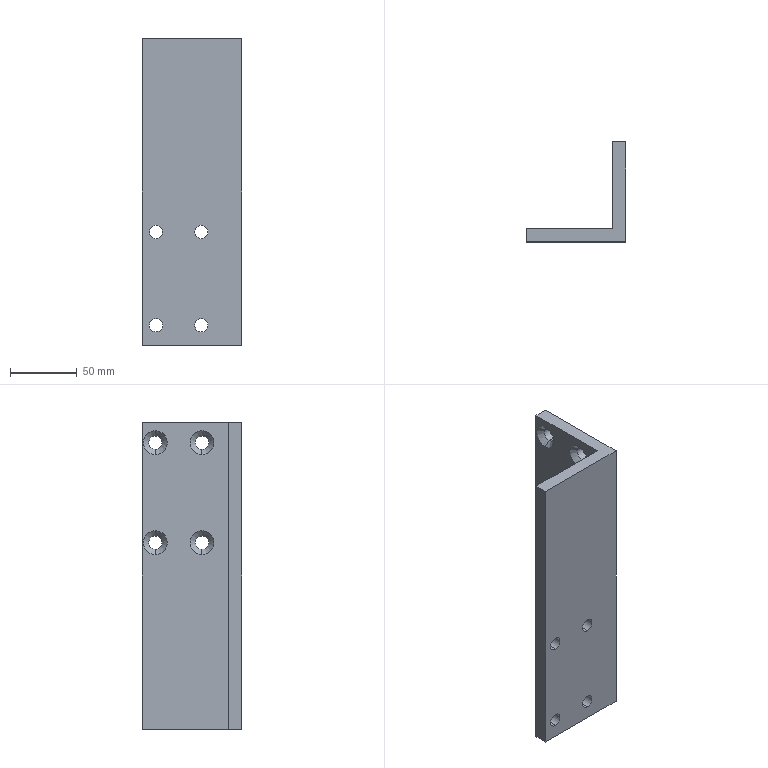Part | SolidWorks | features HoleWzd 2, Extrusion 1, MoveFace 1 | 1 solid | 32 faces | box 75 x 75 x 230 mm | volume 314471 mm3 | cylinder 16 | cone 8 | plane 8 | commonest cylinder face diameters 10 x16
STEP:
#1=CARTESIAN_POINT('',(10.5,0.,-170.));
#2=VERTEX_POINT('',#1);
#3=CARTESIAN_POINT('',(10.5,0.,-160.));
#4=VERTEX_POINT('',#3);
#5=CARTESIAN_POINT('',(10.5,0.,-165.));
#6=DIRECTION('',(0.,1.,0.));
#7=DIRECTION('',(0.,0.,1.));
#8=AXIS2_PLACEMENT_3D('',#5,#6,#7);
#9=CIRCLE('',#8,5.);
#10=EDGE_CURVE('',#2,#4,#9,.T.);
#11=ORIENTED_EDGE('',*,*,#10,.F.);
#12=CARTESIAN_POINT('',(10.5,10.,-170.));
#13=VERTEX_POINT('',#12);
#14=CARTESIAN_POINT('',(10.5,10.,-170.));
#15=DIRECTION('',(0.,1.,0.));
#16=VECTOR('',#15,1000.);
#17=LINE('',#14,#16);
#18=EDGE_CURVE('',#2,#13,#17,.T.);
#19=ORIENTED_EDGE('',*,*,#18,.T.);
#20=CARTESIAN_POINT('',(10.5,10.,-160.));
#21=VERTEX_POINT('',#20);
#22=CARTESIAN_POINT('',(10.5,10.,-165.));
#23=DIRECTION('',(0.,1.,0.));
#24=DIRECTION('',(0.,0.,1.));
#25=AXIS2_PLACEMENT_3D('',#22,#23,#24);
#26=CIRCLE('',#25,5.);
#27=EDGE_CURVE('',#13,#21,#26,.T.);
#28=ORIENTED_EDGE('',*,*,#27,.T.);
#29=CARTESIAN_POINT('',(10.5,10.,-160.));
#30=DIRECTION('',(0.,1.,0.));
#31=VECTOR('',#30,1000.);
#32=LINE('',#29,#31);
#33=EDGE_CURVE('',#4,#21,#32,.T.);
#34=ORIENTED_EDGE('',*,*,#33,.F.);
#35=EDGE_LOOP('',(#11,#19,#28,#34));
#36=FACE_OUTER_BOUND('',#35,.T.);
#37=CARTESIAN_POINT('',(10.5,10.,-165.));
#38=DIRECTION('',(0.,1.,0.));
#39=DIRECTION('',(0.,0.,1.));
#40=AXIS2_PLACEMENT_3D('',#37,#38,#39);
#41=CYLINDRICAL_SURFACE('',#40,5.);
#42=ADVANCED_FACE('',(#36),#41,.F.);
#43=CARTESIAN_POINT('',(10.5,0.,-100.));
#44=VERTEX_POINT('',#43);
#45=CARTESIAN_POINT('',(10.5,0.,-90.));
#46=VERTEX_POINT('',#45);
#47=CARTESIAN_POINT('',(10.5,0.,-95.));
#48=DIRECTION('',(0.,1.,0.));
#49=DIRECTION('',(0.,0.,1.));
#50=AXIS2_PLACEMENT_3D('',#47,#48,#49);
#51=CIRCLE('',#50,5.);
#52=EDGE_CURVE('',#44,#46,#51,.T.);
#53=ORIENTED_EDGE('',*,*,#52,.F.);
#54=CARTESIAN_POINT('',(10.5,10.,-100.));
#55=VERTEX_POINT('',#54);
#56=CARTESIAN_POINT('',(10.5,10.,-100.));
#57=DIRECTION('',(0.,1.,0.));
#58=VECTOR('',#57,1000.);
#59=LINE('',#56,#58);
#60=EDGE_CURVE('',#44,#55,#59,.T.);
#61=ORIENTED_EDGE('',*,*,#60,.T.);
#62=CARTESIAN_POINT('',(10.5,10.,-90.));
#63=VERTEX_POINT('',#62);
#64=CARTESIAN_POINT('',(10.5,10.,-95.));
#65=DIRECTION('',(0.,1.,0.));
#66=DIRECTION('',(0.,0.,1.));
#67=AXIS2_PLACEMENT_3D('',#64,#65,#66);
#68=CIRCLE('',#67,5.);
#69=EDGE_CURVE('',#55,#63,#68,.T.);
#70=ORIENTED_EDGE('',*,*,#69,.T.);
#71=CARTESIAN_POINT('',(10.5,10.,-90.));
#72=DIRECTION('',(0.,1.,0.));
#73=VECTOR('',#72,1000.);
#74=LINE('',#71,#73);
#75=EDGE_CURVE('',#46,#63,#74,.T.);
#76=ORIENTED_EDGE('',*,*,#75,.F.);
#77=EDGE_LOOP('',(#53,#61,#70,#76));
#78=FACE_OUTER_BOUND('',#77,.T.);
#79=CARTESIAN_POINT('',(10.5,10.,-95.));
#80=DIRECTION('',(0.,1.,0.));
#81=DIRECTION('',(0.,0.,1.));
#82=AXIS2_PLACEMENT_3D('',#79,#80,#81);
#83=CYLINDRICAL_SURFACE('',#82,5.);
#84=ADVANCED_FACE('',(#78),#83,.F.);
#85=CARTESIAN_POINT('',(44.5,0.,-170.));
#86=VERTEX_POINT('',#85);
#87=CARTESIAN_POINT('',(44.5,0.,-160.));
#88=VERTEX_POINT('',#87);
#89=CARTESIAN_POINT('',(44.5,0.,-165.));
#90=DIRECTION('',(0.,1.,0.));
#91=DIRECTION('',(0.,0.,1.));
#92=AXIS2_PLACEMENT_3D('',#89,#90,#91);
#93=CIRCLE('',#92,5.);
#94=EDGE_CURVE('',#86,#88,#93,.T.);
#95=ORIENTED_EDGE('',*,*,#94,.F.);
#96=CARTESIAN_POINT('',(44.5,10.,-170.));
#97=VERTEX_POINT('',#96);
#98=CARTESIAN_POINT('',(44.5,10.,-170.));
#99=DIRECTION('',(0.,1.,0.));
#100=VECTOR('',#99,1000.);
#101=LINE('',#98,#100);
#102=EDGE_CURVE('',#86,#97,#101,.T.);
#103=ORIENTED_EDGE('',*,*,#102,.T.);
#104=CARTESIAN_POINT('',(44.5,10.,-160.));
#105=VERTEX_POINT('',#104);
#106=CARTESIAN_POINT('',(44.5,10.,-165.));
#107=DIRECTION('',(0.,1.,0.));
#108=DIRECTION('',(0.,0.,1.));
#109=AXIS2_PLACEMENT_3D('',#106,#107,#108);
#110=CIRCLE('',#109,5.);
#111=EDGE_CURVE('',#97,#105,#110,.T.);
#112=ORIENTED_EDGE('',*,*,#111,.T.);
#113=CARTESIAN_POINT('',(44.5,10.,-160.));
#114=DIRECTION('',(0.,1.,0.));
#115=VECTOR('',#114,1000.);
#116=LINE('',#113,#115);
#117=EDGE_CURVE('',#88,#105,#116,.T.);
#118=ORIENTED_EDGE('',*,*,#117,.F.);
#119=EDGE_LOOP('',(#95,#103,#112,#118));
#120=FACE_OUTER_BOUND('',#119,.T.);
#121=CARTESIAN_POINT('',(44.5,10.,-165.));
#122=DIRECTION('',(0.,1.,0.));
#123=DIRECTION('',(0.,0.,1.));
#124=AXIS2_PLACEMENT_3D('',#121,#122,#123);
#125=CYLINDRICAL_SURFACE('',#124,5.);
#126=ADVANCED_FACE('',(#120),#125,.F.);
#127=CARTESIAN_POINT('',(44.5,0.,-100.));
#128=VERTEX_POINT('',#127);
#129=CARTESIAN_POINT('',(44.5,0.,-90.));
#130=VERTEX_POINT('',#129);
#131=CARTESIAN_POINT('',(44.5,0.,-95.));
#132=DIRECTION('',(0.,1.,0.));
#133=DIRECTION('',(0.,0.,1.));
#134=AXIS2_PLACEMENT_3D('',#131,#132,#133);
#135=CIRCLE('',#134,5.);
#136=EDGE_CURVE('',#128,#130,#135,.T.);
#137=ORIENTED_EDGE('',*,*,#136,.F.);
#138=CARTESIAN_POINT('',(44.5,10.,-100.));
#139=VERTEX_POINT('',#138);
#140=CARTESIAN_POINT('',(44.5,10.,-100.));
#141=DIRECTION('',(0.,1.,0.));
#142=VECTOR('',#141,1000.);
#143=LINE('',#140,#142);
#144=EDGE_CURVE('',#128,#139,#143,.T.);
#145=ORIENTED_EDGE('',*,*,#144,.T.);
#146=CARTESIAN_POINT('',(44.5,10.,-90.));
#147=VERTEX_POINT('',#146);
#148=CARTESIAN_POINT('',(44.5,10.,-95.));
#149=DIRECTION('',(0.,1.,0.));
#150=DIRECTION('',(0.,0.,1.));
#151=AXIS2_PLACEMENT_3D('',#148,#149,#150);
#152=CIRCLE('',#151,5.);
#153=EDGE_CURVE('',#139,#147,#152,.T.);
#154=ORIENTED_EDGE('',*,*,#153,.T.);
#155=CARTESIAN_POINT('',(44.5,10.,-90.));
#156=DIRECTION('',(0.,1.,0.));
#157=VECTOR('',#156,1000.);
#158=LINE('',#155,#157);
#159=EDGE_CURVE('',#130,#147,#158,.T.);
#160=ORIENTED_EDGE('',*,*,#159,.F.);
#161=EDGE_LOOP('',(#137,#145,#154,#160));
#162=FACE_OUTER_BOUND('',#161,.T.);
#163=CARTESIAN_POINT('',(44.5,10.,-95.));
#164=DIRECTION('',(0.,1.,0.));
#165=DIRECTION('',(0.,0.,1.));
#166=AXIS2_PLACEMENT_3D('',#163,#164,#165);
#167=CYLINDRICAL_SURFACE('',#166,5.);
#168=ADVANCED_FACE('',(#162),#167,.F.);
#169=CARTESIAN_POINT('',(68.96,65.,-45.));
#170=VERTEX_POINT('',#169);
#171=CARTESIAN_POINT('',(68.96,65.,-35.));
#172=VERTEX_POINT('',#171);
#173=CARTESIAN_POINT('',(68.96,65.,-40.));
#174=DIRECTION('',(-1.,0.,0.));
#175=DIRECTION('',(0.,0.,1.));
#176=AXIS2_PLACEMENT_3D('',#173,#174,#175);
#177=CIRCLE('',#176,5.);
#178=EDGE_CURVE('',#170,#172,#177,.T.);
#179=ORIENTED_EDGE('',*,*,#178,.F.);
#180=CARTESIAN_POINT('',(65.,65.,-48.96));
#181=VERTEX_POINT('',#180);
#182=CARTESIAN_POINT('',(65.,65.,-48.96));
#183=DIRECTION('',(-0.7071,0.,-0.7071));
#184=VECTOR('',#183,1000.);
#185=LINE('',#182,#184);
#186=EDGE_CURVE('',#170,#181,#185,.T.);
#187=ORIENTED_EDGE('',*,*,#186,.T.);
#188=CARTESIAN_POINT('',(65.,65.,-31.04));
#189=VERTEX_POINT('',#188);
#190=CARTESIAN_POINT('',(65.,65.,-40.));
#191=DIRECTION('',(-1.,0.,0.));
#192=DIRECTION('',(0.,0.,1.));
#193=AXIS2_PLACEMENT_3D('',#190,#191,#192);
#194=CIRCLE('',#193,8.96);
#195=EDGE_CURVE('',#181,#189,#194,.T.);
#196=ORIENTED_EDGE('',*,*,#195,.T.);
#197=CARTESIAN_POINT('',(65.,65.,-31.04));
#198=DIRECTION('',(-0.7071,0.,0.7071));
#199=VECTOR('',#198,1000.);
#200=LINE('',#197,#199);
#201=EDGE_CURVE('',#172,#189,#200,.T.);
#202=ORIENTED_EDGE('',*,*,#201,.F.);
#203=EDGE_LOOP('',(#179,#187,#196,#202));
#204=FACE_OUTER_BOUND('',#203,.T.);
#205=CARTESIAN_POINT('',(65.,65.,-40.));
#206=DIRECTION('',(-1.,0.,0.));
#207=DIRECTION('',(0.,0.,1.));
#208=AXIS2_PLACEMENT_3D('',#205,#206,#207);
#209=CONICAL_SURFACE('',#208,8.96,0.7854);
#210=ADVANCED_FACE('',(#204),#209,.F.);
#211=CARTESIAN_POINT('',(75.,65.,-45.));
#212=VERTEX_POINT('',#211);
#213=CARTESIAN_POINT('',(75.,65.,-35.));
#214=VERTEX_POINT('',#213);
#215=CARTESIAN_POINT('',(75.,65.,-40.));
#216=DIRECTION('',(-1.,0.,0.));
#217=DIRECTION('',(0.,0.,1.));
#218=AXIS2_PLACEMENT_3D('',#215,#216,#217);
#219=CIRCLE('',#218,5.);
#220=EDGE_CURVE('',#212,#214,#219,.T.);
#221=ORIENTED_EDGE('',*,*,#220,.F.);
#222=CARTESIAN_POINT('',(65.,65.,-45.));
#223=DIRECTION('',(-1.,0.,0.));
#224=VECTOR('',#223,1000.);
#225=LINE('',#222,#224);
#226=EDGE_CURVE('',#212,#170,#225,.T.);
#227=ORIENTED_EDGE('',*,*,#226,.T.);
#228=ORIENTED_EDGE('',*,*,#178,.T.);
#229=CARTESIAN_POINT('',(65.,65.,-35.));
#230=DIRECTION('',(-1.,0.,0.));
#231=VECTOR('',#230,1000.);
#232=LINE('',#229,#231);
#233=EDGE_CURVE('',#214,#172,#232,.T.);
#234=ORIENTED_EDGE('',*,*,#233,.F.);
#235=EDGE_LOOP('',(#221,#227,#228,#234));
#236=FACE_OUTER_BOUND('',#235,.T.);
#237=CARTESIAN_POINT('',(65.,65.,-40.));
#238=DIRECTION('',(-1.,0.,0.));
#239=DIRECTION('',(0.,0.,1.));
#240=AXIS2_PLACEMENT_3D('',#237,#238,#239);
#241=CYLINDRICAL_SURFACE('',#240,5.);
#242=ADVANCED_FACE('',(#236),#241,.F.);
#243=CARTESIAN_POINT('',(68.96,65.,30.));
#244=VERTEX_POINT('',#243);
#245=CARTESIAN_POINT('',(68.96,65.,40.));
#246=VERTEX_POINT('',#245);
#247=CARTESIAN_POINT('',(68.96,65.,35.));
#248=DIRECTION('',(-1.,0.,0.));
#249=DIRECTION('',(0.,0.,1.));
#250=AXIS2_PLACEMENT_3D('',#247,#248,#249);
#251=CIRCLE('',#250,5.);
#252=EDGE_CURVE('',#244,#246,#251,.T.);
#253=ORIENTED_EDGE('',*,*,#252,.F.);
#254=CARTESIAN_POINT('',(65.,65.,26.04));
#255=VERTEX_POINT('',#254);
#256=CARTESIAN_POINT('',(65.,65.,26.04));
#257=DIRECTION('',(-0.7071,0.,-0.7071));
#258=VECTOR('',#257,1000.);
#259=LINE('',#256,#258);
#260=EDGE_CURVE('',#244,#255,#259,.T.);
#261=ORIENTED_EDGE('',*,*,#260,.T.);
#262=CARTESIAN_POINT('',(65.,65.,43.96));
#263=VERTEX_POINT('',#262);
#264=CARTESIAN_POINT('',(65.,65.,35.));
#265=DIRECTION('',(-1.,0.,0.));
#266=DIRECTION('',(0.,0.,1.));
#267=AXIS2_PLACEMENT_3D('',#264,#265,#266);
#268=CIRCLE('',#267,8.96);
#269=EDGE_CURVE('',#255,#263,#268,.T.);
#270=ORIENTED_EDGE('',*,*,#269,.T.);
#271=CARTESIAN_POINT('',(65.,65.,43.96));
#272=DIRECTION('',(-0.7071,0.,0.7071));
#273=VECTOR('',#272,1000.);
#274=LINE('',#271,#273);
#275=EDGE_CURVE('',#246,#263,#274,.T.);
#276=ORIENTED_EDGE('',*,*,#275,.F.);
#277=EDGE_LOOP('',(#253,#261,#270,#276));
#278=FACE_OUTER_BOUND('',#277,.T.);
#279=CARTESIAN_POINT('',(65.,65.,35.));
#280=DIRECTION('',(-1.,0.,0.));
#281=DIRECTION('',(0.,0.,1.));
#282=AXIS2_PLACEMENT_3D('',#279,#280,#281);
#283=CONICAL_SURFACE('',#282,8.96,0.7854);
#284=ADVANCED_FACE('',(#278),#283,.F.);
#285=CARTESIAN_POINT('',(75.,65.,30.));
#286=VERTEX_POINT('',#285);
#287=CARTESIAN_POINT('',(75.,65.,40.));
#288=VERTEX_POINT('',#287);
#289=CARTESIAN_POINT('',(75.,65.,35.));
#290=DIRECTION('',(-1.,0.,0.));
#291=DIRECTION('',(0.,0.,1.));
#292=AXIS2_PLACEMENT_3D('',#289,#290,#291);
#293=CIRCLE('',#292,5.);
#294=EDGE_CURVE('',#286,#288,#293,.T.);
#295=ORIENTED_EDGE('',*,*,#294,.F.);
#296=CARTESIAN_POINT('',(65.,65.,30.));
#297=DIRECTION('',(-1.,0.,0.));
#298=VECTOR('',#297,1000.);
#299=LINE('',#296,#298);
#300=EDGE_CURVE('',#286,#244,#299,.T.);
#301=ORIENTED_EDGE('',*,*,#300,.T.);
#302=ORIENTED_EDGE('',*,*,#252,.T.);
#303=CARTESIAN_POINT('',(65.,65.,40.));
#304=DIRECTION('',(-1.,0.,0.));
#305=VECTOR('',#304,1000.);
#306=LINE('',#303,#305);
#307=EDGE_CURVE('',#288,#246,#306,.T.);
#308=ORIENTED_EDGE('',*,*,#307,.F.);
#309=EDGE_LOOP('',(#295,#301,#302,#308));
#310=FACE_OUTER_BOUND('',#309,.T.);
#311=CARTESIAN_POINT('',(65.,65.,35.));
#312=DIRECTION('',(-1.,0.,0.));
#313=DIRECTION('',(0.,0.,1.));
#314=AXIS2_PLACEMENT_3D('',#311,#312,#313);
#315=CYLINDRICAL_SURFACE('',#314,5.);
#316=ADVANCED_FACE('',(#310),#315,.F.);
#317=CARTESIAN_POINT('',(68.96,30.,-45.));
#318=VERTEX_POINT('',#317);
#319=CARTESIAN_POINT('',(68.96,30.,-35.));
#320=VERTEX_POINT('',#319);
#321=CARTESIAN_POINT('',(68.96,30.,-40.));
#322=DIRECTION('',(-1.,0.,0.));
#323=DIRECTION('',(0.,0.,1.));
#324=AXIS2_PLACEMENT_3D('',#321,#322,#323);
#325=CIRCLE('',#324,5.);
#326=EDGE_CURVE('',#318,#320,#325,.T.);
#327=ORIENTED_EDGE('',*,*,#326,.F.);
#328=CARTESIAN_POINT('',(65.,30.,-48.96));
#329=VERTEX_POINT('',#328);
#330=CARTESIAN_POINT('',(65.,30.,-48.96));
#331=DIRECTION('',(-0.7071,0.,-0.7071));
#332=VECTOR('',#331,1000.);
#333=LINE('',#330,#332);
#334=EDGE_CURVE('',#318,#329,#333,.T.);
#335=ORIENTED_EDGE('',*,*,#334,.T.);
#336=CARTESIAN_POINT('',(65.,30.,-31.04));
#337=VERTEX_POINT('',#336);
#338=CARTESIAN_POINT('',(65.,30.,-40.));
#339=DIRECTION('',(-1.,0.,0.));
#340=DIRECTION('',(0.,0.,1.));
#341=AXIS2_PLACEMENT_3D('',#338,#339,#340);
#342=CIRCLE('',#341,8.96);
#343=EDGE_CURVE('',#329,#337,#342,.T.);
#344=ORIENTED_EDGE('',*,*,#343,.T.);
#345=CARTESIAN_POINT('',(65.,30.,-31.04));
#346=DIRECTION('',(-0.7071,0.,0.7071));
#347=VECTOR('',#346,1000.);
#348=LINE('',#345,#347);
#349=EDGE_CURVE('',#320,#337,#348,.T.);
#350=ORIENTED_EDGE('',*,*,#349,.F.);
#351=EDGE_LOOP('',(#327,#335,#344,#350));
#352=FACE_OUTER_BOUND('',#351,.T.);
#353=CARTESIAN_POINT('',(65.,30.,-40.));
#354=DIRECTION('',(-1.,0.,0.));
#355=DIRECTION('',(0.,0.,1.));
#356=AXIS2_PLACEMENT_3D('',#353,#354,#355);
#357=CONICAL_SURFACE('',#356,8.96,0.7854);
#358=ADVANCED_FACE('',(#352),#357,.F.);
#359=CARTESIAN_POINT('',(75.,30.,-45.));
#360=VERTEX_POINT('',#359);
#361=CARTESIAN_POINT('',(75.,30.,-35.));
#362=VERTEX_POINT('',#361);
#363=CARTESIAN_POINT('',(75.,30.,-40.));
#364=DIRECTION('',(-1.,0.,0.));
#365=DIRECTION('',(0.,0.,1.));
#366=AXIS2_PLACEMENT_3D('',#363,#364,#365);
#367=CIRCLE('',#366,5.);
#368=EDGE_CURVE('',#360,#362,#367,.T.);
#369=ORIENTED_EDGE('',*,*,#368,.F.);
#370=CARTESIAN_POINT('',(65.,30.,-45.));
#371=DIRECTION('',(-1.,0.,0.));
#372=VECTOR('',#371,1000.);
#373=LINE('',#370,#372);
#374=EDGE_CURVE('',#360,#318,#373,.T.);
#375=ORIENTED_EDGE('',*,*,#374,.T.);
#376=ORIENTED_EDGE('',*,*,#326,.T.);
#377=CARTESIAN_POINT('',(65.,30.,-35.));
#378=DIRECTION('',(-1.,0.,0.));
#379=VECTOR('',#378,1000.);
#380=LINE('',#377,#379);
#381=EDGE_CURVE('',#362,#320,#380,.T.);
#382=ORIENTED_EDGE('',*,*,#381,.F.);
#383=EDGE_LOOP('',(#369,#375,#376,#382));
#384=FACE_OUTER_BOUND('',#383,.T.);
#385=CARTESIAN_POINT('',(65.,30.,-40.));
#386=DIRECTION('',(-1.,0.,0.));
#387=DIRECTION('',(0.,0.,1.));
#388=AXIS2_PLACEMENT_3D('',#385,#386,#387);
#389=CYLINDRICAL_SURFACE('',#388,5.);
#390=ADVANCED_FACE('',(#384),#389,.F.);
#391=CARTESIAN_POINT('',(68.96,30.,30.));
#392=VERTEX_POINT('',#391);
#393=CARTESIAN_POINT('',(68.96,30.,40.));
#394=VERTEX_POINT('',#393);
#395=CARTESIAN_POINT('',(68.96,30.,35.));
#396=DIRECTION('',(-1.,0.,0.));
#397=DIRECTION('',(0.,0.,1.));
#398=AXIS2_PLACEMENT_3D('',#395,#396,#397);
#399=CIRCLE('',#398,5.);
#400=EDGE_CURVE('',#392,#394,#399,.T.);
#401=ORIENTED_EDGE('',*,*,#400,.F.);
#402=CARTESIAN_POINT('',(65.,30.,26.04));
#403=VERTEX_POINT('',#402);
#404=CARTESIAN_POINT('',(65.,30.,26.04));
#405=DIRECTION('',(-0.7071,0.,-0.7071));
#406=VECTOR('',#405,1000.);
#407=LINE('',#404,#406);
#408=EDGE_CURVE('',#392,#403,#407,.T.);
#409=ORIENTED_EDGE('',*,*,#408,.T.);
#410=CARTESIAN_POINT('',(65.,30.,43.96));
#411=VERTEX_POINT('',#410);
#412=CARTESIAN_POINT('',(65.,30.,35.));
#413=DIRECTION('',(-1.,0.,0.));
#414=DIRECTION('',(0.,0.,1.));
#415=AXIS2_PLACEMENT_3D('',#412,#413,#414);
#416=CIRCLE('',#415,8.96);
#417=EDGE_CURVE('',#403,#411,#416,.T.);
#418=ORIENTED_EDGE('',*,*,#417,.T.);
#419=CARTESIAN_POINT('',(65.,30.,43.96));
#420=DIRECTION('',(-0.7071,0.,0.7071));
#421=VECTOR('',#420,1000.);
#422=LINE('',#419,#421);
#423=EDGE_CURVE('',#394,#411,#422,.T.);
#424=ORIENTED_EDGE('',*,*,#423,.F.);
#425=EDGE_LOOP('',(#401,#409,#418,#424));
#426=FACE_OUTER_BOUND('',#425,.T.);
#427=CARTESIAN_POINT('',(65.,30.,35.));
#428=DIRECTION('',(-1.,0.,0.));
#429=DIRECTION('',(0.,0.,1.));
#430=AXIS2_PLACEMENT_3D('',#427,#428,#429);
#431=CONICAL_SURFACE('',#430,8.96,0.7854);
#432=ADVANCED_FACE('',(#426),#431,.F.);
#433=CARTESIAN_POINT('',(75.,30.,30.));
#434=VERTEX_POINT('',#433);
#435=CARTESIAN_POINT('',(75.,30.,40.));
#436=VERTEX_POINT('',#435);
#437=CARTESIAN_POINT('',(75.,30.,35.));
#438=DIRECTION('',(-1.,0.,0.));
#439=DIRECTION('',(0.,0.,1.));
#440=AXIS2_PLACEMENT_3D('',#437,#438,#439);
#441=CIRCLE('',#440,5.);
#442=EDGE_CURVE('',#434,#436,#441,.T.);
#443=ORIENTED_EDGE('',*,*,#442,.F.);
#444=CARTESIAN_POINT('',(65.,30.,30.));
#445=DIRECTION('',(-1.,0.,0.));
#446=VECTOR('',#445,1000.);
#447=LINE('',#444,#446);
#448=EDGE_CURVE('',#434,#392,#447,.T.);
#449=ORIENTED_EDGE('',*,*,#448,.T.);
#450=ORIENTED_EDGE('',*,*,#400,.T.);
#451=CARTESIAN_POINT('',(65.,30.,40.));
#452=DIRECTION('',(-1.,0.,0.));
#453=VECTOR('',#452,1000.);
#454=LINE('',#451,#453);
#455=EDGE_CURVE('',#436,#394,#454,.T.);
#456=ORIENTED_EDGE('',*,*,#455,.F.);
#457=EDGE_LOOP('',(#443,#449,#450,#456));
#458=FACE_OUTER_BOUND('',#457,.T.);
#459=CARTESIAN_POINT('',(65.,30.,35.));
#460=DIRECTION('',(-1.,0.,0.));
#461=DIRECTION('',(0.,0.,1.));
#462=AXIS2_PLACEMENT_3D('',#459,#460,#461);
#463=CYLINDRICAL_SURFACE('',#462,5.);
#464=ADVANCED_FACE('',(#458),#463,.F.);
#465=CARTESIAN_POINT('',(10.5,10.,-165.));
#466=DIRECTION('',(0.,1.,0.));
#467=DIRECTION('',(0.,0.,1.));
#468=AXIS2_PLACEMENT_3D('',#465,#466,#467);
#469=CIRCLE('',#468,5.);
#470=EDGE_CURVE('',#21,#13,#469,.T.);
#471=ORIENTED_EDGE('',*,*,#470,.F.);
#472=ORIENTED_EDGE('',*,*,#27,.F.);
#473=EDGE_LOOP('',(#471,#472));
#474=FACE_BOUND('',#473,.T.);
#475=CARTESIAN_POINT('',(10.5,10.,-95.));
#476=DIRECTION('',(0.,1.,0.));
#477=DIRECTION('',(0.,0.,1.));
#478=AXIS2_PLACEMENT_3D('',#475,#476,#477);
#479=CIRCLE('',#478,5.);
#480=EDGE_CURVE('',#63,#55,#479,.T.);
#481=ORIENTED_EDGE('',*,*,#480,.F.);
#482=ORIENTED_EDGE('',*,*,#69,.F.);
#483=EDGE_LOOP('',(#481,#482));
#484=FACE_BOUND('',#483,.T.);
#485=CARTESIAN_POINT('',(44.5,10.,-165.));
#486=DIRECTION('',(0.,1.,0.));
#487=DIRECTION('',(0.,0.,1.));
#488=AXIS2_PLACEMENT_3D('',#485,#486,#487);
#489=CIRCLE('',#488,5.);
#490=EDGE_CURVE('',#105,#97,#489,.T.);
#491=ORIENTED_EDGE('',*,*,#490,.F.);
#492=ORIENTED_EDGE('',*,*,#111,.F.);
#493=EDGE_LOOP('',(#491,#492));
#494=FACE_BOUND('',#493,.T.);
#495=CARTESIAN_POINT('',(65.,10.,-180.));
#496=VERTEX_POINT('',#495);
#497=CARTESIAN_POINT('',(0.,10.,-180.));
#498=VERTEX_POINT('',#497);
#499=CARTESIAN_POINT('',(65.,10.,-180.));
#500=DIRECTION('',(-1.,0.,0.));
#501=VECTOR('',#500,1000.);
#502=LINE('',#499,#501);
#503=EDGE_CURVE('',#496,#498,#502,.T.);
#504=ORIENTED_EDGE('',*,*,#503,.T.);
#505=CARTESIAN_POINT('',(0.,10.,50.));
#506=VERTEX_POINT('',#505);
#507=CARTESIAN_POINT('',(0.,10.,50.));
#508=DIRECTION('',(0.,0.,-1.));
#509=VECTOR('',#508,1000.);
#510=LINE('',#507,#509);
#511=EDGE_CURVE('',#506,#498,#510,.T.);
#512=ORIENTED_EDGE('',*,*,#511,.F.);
#513=CARTESIAN_POINT('',(65.,10.,50.));
#514=VERTEX_POINT('',#513);
#515=CARTESIAN_POINT('',(65.,10.,50.));
#516=DIRECTION('',(-1.,0.,0.));
#517=VECTOR('',#516,1000.);
#518=LINE('',#515,#517);
#519=EDGE_CURVE('',#514,#506,#518,.T.);
#520=ORIENTED_EDGE('',*,*,#519,.F.);
#521=CARTESIAN_POINT('',(65.,10.,50.));
#522=DIRECTION('',(0.,0.,-1.));
#523=VECTOR('',#522,1000.);
#524=LINE('',#521,#523);
#525=EDGE_CURVE('',#514,#496,#524,.T.);
#526=ORIENTED_EDGE('',*,*,#525,.T.);
#527=EDGE_LOOP('',(#504,#512,#520,#526));
#528=FACE_OUTER_BOUND('',#527,.T.);
#529=CARTESIAN_POINT('',(44.5,10.,-95.));
#530=DIRECTION('',(0.,1.,0.));
#531=DIRECTION('',(0.,0.,1.));
#532=AXIS2_PLACEMENT_3D('',#529,#530,#531);
#533=CIRCLE('',#532,5.);
#534=EDGE_CURVE('',#147,#139,#533,.T.);
#535=ORIENTED_EDGE('',*,*,#534,.F.);
#536=ORIENTED_EDGE('',*,*,#153,.F.);
#537=EDGE_LOOP('',(#535,#536));
#538=FACE_BOUND('',#537,.T.);
#539=CARTESIAN_POINT('',(65.,10.,50.));
#540=DIRECTION('',(0.,-1.,0.));
#541=DIRECTION('',(1.,0.,0.));
#542=AXIS2_PLACEMENT_3D('',#539,#540,#541);
#543=PLANE('',#542);
#544=ADVANCED_FACE('',(#474,#484,#494,#528,#538),#543,.F.);
#545=CARTESIAN_POINT('',(0.,0.,-180.));
#546=VERTEX_POINT('',#545);
#547=CARTESIAN_POINT('',(0.,10.,-180.));
#548=DIRECTION('',(0.,-1.,0.));
#549=VECTOR('',#548,1000.);
#550=LINE('',#547,#549);
#551=EDGE_CURVE('',#498,#546,#550,.T.);
#552=ORIENTED_EDGE('',*,*,#551,.T.);
#553=CARTESIAN_POINT('',(0.,0.,50.));
#554=VERTEX_POINT('',#553);
#555=CARTESIAN_POINT('',(0.,0.,50.));
#556=DIRECTION('',(0.,0.,-1.));
#557=VECTOR('',#556,1000.);
#558=LINE('',#555,#557);
#559=EDGE_CURVE('',#554,#546,#558,.T.);
#560=ORIENTED_EDGE('',*,*,#559,.F.);
#561=CARTESIAN_POINT('',(0.,10.,50.));
#562=DIRECTION('',(0.,-1.,0.));
#563=VECTOR('',#562,1000.);
#564=LINE('',#561,#563);
#565=EDGE_CURVE('',#506,#554,#564,.T.);
#566=ORIENTED_EDGE('',*,*,#565,.F.);
#567=ORIENTED_EDGE('',*,*,#511,.T.);
#568=EDGE_LOOP('',(#552,#560,#566,#567));
#569=FACE_OUTER_BOUND('',#568,.T.);
#570=CARTESIAN_POINT('',(0.,10.,50.));
#571=DIRECTION('',(1.,0.,0.));
#572=DIRECTION('',(0.,1.,0.));
#573=AXIS2_PLACEMENT_3D('',#570,#571,#572);
#574=PLANE('',#573);
#575=ADVANCED_FACE('',(#569),#574,.F.);
#576=CARTESIAN_POINT('',(10.5,0.,-165.));
#577=DIRECTION('',(0.,1.,0.));
#578=DIRECTION('',(0.,0.,1.));
#579=AXIS2_PLACEMENT_3D('',#576,#577,#578);
#580=CIRCLE('',#579,5.);
#581=EDGE_CURVE('',#4,#2,#580,.T.);
#582=ORIENTED_EDGE('',*,*,#581,.T.);
#583=ORIENTED_EDGE('',*,*,#10,.T.);
#584=EDGE_LOOP('',(#582,#583));
#585=FACE_BOUND('',#584,.T.);
#586=CARTESIAN_POINT('',(10.5,0.,-95.));
#587=DIRECTION('',(0.,1.,0.));
#588=DIRECTION('',(0.,0.,1.));
#589=AXIS2_PLACEMENT_3D('',#586,#587,#588);
#590=CIRCLE('',#589,5.);
#591=EDGE_CURVE('',#46,#44,#590,.T.);
#592=ORIENTED_EDGE('',*,*,#591,.T.);
#593=ORIENTED_EDGE('',*,*,#52,.T.);
#594=EDGE_LOOP('',(#592,#593));
#595=FACE_BOUND('',#594,.T.);
#596=CARTESIAN_POINT('',(44.5,0.,-165.));
#597=DIRECTION('',(0.,1.,0.));
#598=DIRECTION('',(0.,0.,1.));
#599=AXIS2_PLACEMENT_3D('',#596,#597,#598);
#600=CIRCLE('',#599,5.);
#601=EDGE_CURVE('',#88,#86,#600,.T.);
#602=ORIENTED_EDGE('',*,*,#601,.T.);
#603=ORIENTED_EDGE('',*,*,#94,.T.);
#604=EDGE_LOOP('',(#602,#603));
#605=FACE_BOUND('',#604,.T.);
#606=CARTESIAN_POINT('',(44.5,0.,-95.));
#607=DIRECTION('',(0.,1.,0.));
#608=DIRECTION('',(0.,0.,1.));
#609=AXIS2_PLACEMENT_3D('',#606,#607,#608);
#610=CIRCLE('',#609,5.);
#611=EDGE_CURVE('',#130,#128,#610,.T.);
#612=ORIENTED_EDGE('',*,*,#611,.T.);
#613=ORIENTED_EDGE('',*,*,#136,.T.);
#614=EDGE_LOOP('',(#612,#613));
#615=FACE_BOUND('',#614,.T.);
#616=CARTESIAN_POINT('',(75.,0.,-180.));
#617=VERTEX_POINT('',#616);
#618=CARTESIAN_POINT('',(0.,0.,-180.));
#619=DIRECTION('',(1.,0.,0.));
#620=VECTOR('',#619,1000.);
#621=LINE('',#618,#620);
#622=EDGE_CURVE('',#546,#617,#621,.T.);
#623=ORIENTED_EDGE('',*,*,#622,.T.);
#624=CARTESIAN_POINT('',(75.,0.,50.));
#625=VERTEX_POINT('',#624);
#626=CARTESIAN_POINT('',(75.,0.,50.));
#627=DIRECTION('',(0.,0.,-1.));
#628=VECTOR('',#627,1000.);
#629=LINE('',#626,#628);
#630=EDGE_CURVE('',#625,#617,#629,.T.);
#631=ORIENTED_EDGE('',*,*,#630,.F.);
#632=CARTESIAN_POINT('',(0.,0.,50.));
#633=DIRECTION('',(1.,0.,0.));
#634=VECTOR('',#633,1000.);
#635=LINE('',#632,#634);
#636=EDGE_CURVE('',#554,#625,#635,.T.);
#637=ORIENTED_EDGE('',*,*,#636,.F.);
#638=ORIENTED_EDGE('',*,*,#559,.T.);
#639=EDGE_LOOP('',(#623,#631,#637,#638));
#640=FACE_OUTER_BOUND('',#639,.T.);
#641=CARTESIAN_POINT('',(0.,0.,50.));
#642=DIRECTION('',(0.,1.,0.));
#643=DIRECTION('',(0.,0.,1.));
#644=AXIS2_PLACEMENT_3D('',#641,#642,#643);
#645=PLANE('',#644);
#646=ADVANCED_FACE('',(#585,#595,#605,#615,#640),#645,.F.);
#647=CARTESIAN_POINT('',(75.,65.,-40.));
#648=DIRECTION('',(-1.,0.,0.));
#649=DIRECTION('',(0.,0.,1.));
#650=AXIS2_PLACEMENT_3D('',#647,#648,#649);
#651=CIRCLE('',#650,5.);
#652=EDGE_CURVE('',#214,#212,#651,.T.);
#653=ORIENTED_EDGE('',*,*,#652,.T.);
#654=ORIENTED_EDGE('',*,*,#220,.T.);
#655=EDGE_LOOP('',(#653,#654));
#656=FACE_BOUND('',#655,.T.);
#657=CARTESIAN_POINT('',(75.,65.,35.));
#658=DIRECTION('',(-1.,0.,0.));
#659=DIRECTION('',(0.,0.,1.));
#660=AXIS2_PLACEMENT_3D('',#657,#658,#659);
#661=CIRCLE('',#660,5.);
#662=EDGE_CURVE('',#288,#286,#661,.T.);
#663=ORIENTED_EDGE('',*,*,#662,.T.);
#664=ORIENTED_EDGE('',*,*,#294,.T.);
#665=EDGE_LOOP('',(#663,#664));
#666=FACE_BOUND('',#665,.T.);
#667=CARTESIAN_POINT('',(75.,30.,-40.));
#668=DIRECTION('',(-1.,0.,0.));
#669=DIRECTION('',(0.,0.,1.));
#670=AXIS2_PLACEMENT_3D('',#667,#668,#669);
#671=CIRCLE('',#670,5.);
#672=EDGE_CURVE('',#362,#360,#671,.T.);
#673=ORIENTED_EDGE('',*,*,#672,.T.);
#674=ORIENTED_EDGE('',*,*,#368,.T.);
#675=EDGE_LOOP('',(#673,#674));
#676=FACE_BOUND('',#675,.T.);
#677=CARTESIAN_POINT('',(75.,30.,35.));
#678=DIRECTION('',(-1.,0.,0.));
#679=DIRECTION('',(0.,0.,1.));
#680=AXIS2_PLACEMENT_3D('',#677,#678,#679);
#681=CIRCLE('',#680,5.);
#682=EDGE_CURVE('',#436,#434,#681,.T.);
#683=ORIENTED_EDGE('',*,*,#682,.T.);
#684=ORIENTED_EDGE('',*,*,#442,.T.);
#685=EDGE_LOOP('',(#683,#684));
#686=FACE_BOUND('',#685,.T.);
#687=CARTESIAN_POINT('',(75.,75.,-180.));
#688=VERTEX_POINT('',#687);
#689=CARTESIAN_POINT('',(75.,0.,-180.));
#690=DIRECTION('',(0.,1.,0.));
#691=VECTOR('',#690,1000.);
#692=LINE('',#689,#691);
#693=EDGE_CURVE('',#617,#688,#692,.T.);
#694=ORIENTED_EDGE('',*,*,#693,.T.);
#695=CARTESIAN_POINT('',(75.,75.,50.));
#696=VERTEX_POINT('',#695);
#697=CARTESIAN_POINT('',(75.,75.,50.));
#698=DIRECTION('',(0.,0.,-1.));
#699=VECTOR('',#698,1000.);
#700=LINE('',#697,#699);
#701=EDGE_CURVE('',#696,#688,#700,.T.);
#702=ORIENTED_EDGE('',*,*,#701,.F.);
#703=CARTESIAN_POINT('',(75.,0.,50.));
#704=DIRECTION('',(0.,1.,0.));
#705=VECTOR('',#704,1000.);
#706=LINE('',#703,#705);
#707=EDGE_CURVE('',#625,#696,#706,.T.);
#708=ORIENTED_EDGE('',*,*,#707,.F.);
#709=ORIENTED_EDGE('',*,*,#630,.T.);
#710=EDGE_LOOP('',(#694,#702,#708,#709));
#711=FACE_OUTER_BOUND('',#710,.T.);
#712=CARTESIAN_POINT('',(75.,0.,50.));
#713=DIRECTION('',(-1.,0.,0.));
#714=DIRECTION('',(0.,0.,1.));
#715=AXIS2_PLACEMENT_3D('',#712,#713,#714);
#716=PLANE('',#715);
#717=ADVANCED_FACE('',(#656,#666,#676,#686,#711),#716,.F.);
#718=CARTESIAN_POINT('',(65.,75.,-180.));
#719=VERTEX_POINT('',#718);
#720=CARTESIAN_POINT('',(75.,75.,-180.));
#721=DIRECTION('',(-1.,0.,0.));
#722=VECTOR('',#721,1000.);
#723=LINE('',#720,#722);
#724=EDGE_CURVE('',#688,#719,#723,.T.);
#725=ORIENTED_EDGE('',*,*,#724,.T.);
#726=CARTESIAN_POINT('',(65.,75.,50.));
#727=VERTEX_POINT('',#726);
#728=CARTESIAN_POINT('',(65.,75.,50.));
#729=DIRECTION('',(0.,0.,-1.));
#730=VECTOR('',#729,1000.);
#731=LINE('',#728,#730);
#732=EDGE_CURVE('',#727,#719,#731,.T.);
#733=ORIENTED_EDGE('',*,*,#732,.F.);
#734=CARTESIAN_POINT('',(75.,75.,50.));
#735=DIRECTION('',(-1.,0.,0.));
#736=VECTOR('',#735,1000.);
#737=LINE('',#734,#736);
#738=EDGE_CURVE('',#696,#727,#737,.T.);
#739=ORIENTED_EDGE('',*,*,#738,.F.);
#740=ORIENTED_EDGE('',*,*,#701,.T.);
#741=EDGE_LOOP('',(#725,#733,#739,#740));
#742=FACE_OUTER_BOUND('',#741,.T.);
#743=CARTESIAN_POINT('',(75.,75.,50.));
#744=DIRECTION('',(0.,-1.,0.));
#745=DIRECTION('',(0.,0.,-1.));
#746=AXIS2_PLACEMENT_3D('',#743,#744,#745);
#747=PLANE('',#746);
#748=ADVANCED_FACE('',(#742),#747,.F.);
#749=CARTESIAN_POINT('',(65.,65.,-40.));
#750=DIRECTION('',(-1.,0.,0.));
#751=DIRECTION('',(0.,0.,1.));
#752=AXIS2_PLACEMENT_3D('',#749,#750,#751);
#753=CIRCLE('',#752,8.96);
#754=EDGE_CURVE('',#189,#181,#753,.T.);
#755=ORIENTED_EDGE('',*,*,#754,.F.);
#756=ORIENTED_EDGE('',*,*,#195,.F.);
#757=EDGE_LOOP('',(#755,#756));
#758=FACE_BOUND('',#757,.T.);
#759=CARTESIAN_POINT('',(65.,65.,35.));
#760=DIRECTION('',(-1.,0.,0.));
#761=DIRECTION('',(0.,0.,1.));
#762=AXIS2_PLACEMENT_3D('',#759,#760,#761);
#763=CIRCLE('',#762,8.96);
#764=EDGE_CURVE('',#263,#255,#763,.T.);
#765=ORIENTED_EDGE('',*,*,#764,.F.);
#766=ORIENTED_EDGE('',*,*,#269,.F.);
#767=EDGE_LOOP('',(#765,#766));
#768=FACE_BOUND('',#767,.T.);
#769=CARTESIAN_POINT('',(65.,30.,-40.));
#770=DIRECTION('',(-1.,0.,0.));
#771=DIRECTION('',(0.,0.,1.));
#772=AXIS2_PLACEMENT_3D('',#769,#770,#771);
#773=CIRCLE('',#772,8.96);
#774=EDGE_CURVE('',#337,#329,#773,.T.);
#775=ORIENTED_EDGE('',*,*,#774,.F.);
#776=ORIENTED_EDGE('',*,*,#343,.F.);
#777=EDGE_LOOP('',(#775,#776));
#778=FACE_BOUND('',#777,.T.);
#779=CARTESIAN_POINT('',(65.,30.,35.));
#780=DIRECTION('',(-1.,0.,0.));
#781=DIRECTION('',(0.,0.,1.));
#782=AXIS2_PLACEMENT_3D('',#779,#780,#781);
#783=CIRCLE('',#782,8.96);
#784=EDGE_CURVE('',#411,#403,#783,.T.);
#785=ORIENTED_EDGE('',*,*,#784,.F.);
#786=ORIENTED_EDGE('',*,*,#417,.F.);
#787=EDGE_LOOP('',(#785,#786));
#788=FACE_BOUND('',#787,.T.);
#789=CARTESIAN_POINT('',(65.,75.,-180.));
#790=DIRECTION('',(0.,-1.,0.));
#791=VECTOR('',#790,1000.);
#792=LINE('',#789,#791);
#793=EDGE_CURVE('',#719,#496,#792,.T.);
#794=ORIENTED_EDGE('',*,*,#793,.T.);
#795=ORIENTED_EDGE('',*,*,#525,.F.);
#796=CARTESIAN_POINT('',(65.,75.,50.));
#797=DIRECTION('',(0.,-1.,0.));
#798=VECTOR('',#797,1000.);
#799=LINE('',#796,#798);
#800=EDGE_CURVE('',#727,#514,#799,.T.);
#801=ORIENTED_EDGE('',*,*,#800,.F.);
#802=ORIENTED_EDGE('',*,*,#732,.T.);
#803=EDGE_LOOP('',(#794,#795,#801,#802));
#804=FACE_OUTER_BOUND('',#803,.T.);
#805=CARTESIAN_POINT('',(65.,75.,50.));
#806=DIRECTION('',(1.,0.,0.));
#807=DIRECTION('',(0.,0.,-1.));
#808=AXIS2_PLACEMENT_3D('',#805,#806,#807);
#809=PLANE('',#808);
#810=ADVANCED_FACE('',(#758,#768,#778,#788,#804),#809,.F.);
#811=ORIENTED_EDGE('',*,*,#565,.T.);
#812=ORIENTED_EDGE('',*,*,#636,.T.);
#813=ORIENTED_EDGE('',*,*,#707,.T.);
#814=ORIENTED_EDGE('',*,*,#738,.T.);
#815=ORIENTED_EDGE('',*,*,#800,.T.);
#816=ORIENTED_EDGE('',*,*,#519,.T.);
#817=EDGE_LOOP('',(#811,#812,#813,#814,#815,#816));
#818=FACE_OUTER_BOUND('',#817,.T.);
#819=CARTESIAN_POINT('',(0.,0.,50.));
#820=DIRECTION('',(0.,0.,1.));
#821=DIRECTION('',(1.,0.,0.));
#822=AXIS2_PLACEMENT_3D('',#819,#820,#821);
#823=PLANE('',#822);
#824=ADVANCED_FACE('',(#818),#823,.T.);
#825=ORIENTED_EDGE('',*,*,#551,.F.);
#826=ORIENTED_EDGE('',*,*,#503,.F.);
#827=ORIENTED_EDGE('',*,*,#793,.F.);
#828=ORIENTED_EDGE('',*,*,#724,.F.);
#829=ORIENTED_EDGE('',*,*,#693,.F.);
#830=ORIENTED_EDGE('',*,*,#622,.F.);
#831=EDGE_LOOP('',(#825,#826,#827,#828,#829,#830));
#832=FACE_OUTER_BOUND('',#831,.T.);
#833=CARTESIAN_POINT('',(0.,0.,-180.));
#834=DIRECTION('',(0.,0.,1.));
#835=DIRECTION('',(1.,0.,0.));
#836=AXIS2_PLACEMENT_3D('',#833,#834,#835);
#837=PLANE('',#836);
#838=ADVANCED_FACE('',(#832),#837,.F.);
#839=ORIENTED_EDGE('',*,*,#448,.F.);
#840=ORIENTED_EDGE('',*,*,#682,.F.);
#841=ORIENTED_EDGE('',*,*,#455,.T.);
#842=CARTESIAN_POINT('',(68.96,30.,35.));
#843=DIRECTION('',(-1.,0.,0.));
#844=DIRECTION('',(0.,0.,1.));
#845=AXIS2_PLACEMENT_3D('',#842,#843,#844);
#846=CIRCLE('',#845,5.);
#847=EDGE_CURVE('',#394,#392,#846,.T.);
#848=ORIENTED_EDGE('',*,*,#847,.T.);
#849=EDGE_LOOP('',(#839,#840,#841,#848));
#850=FACE_OUTER_BOUND('',#849,.T.);
#851=CARTESIAN_POINT('',(65.,30.,35.));
#852=DIRECTION('',(-1.,0.,0.));
#853=DIRECTION('',(0.,0.,1.));
#854=AXIS2_PLACEMENT_3D('',#851,#852,#853);
#855=CYLINDRICAL_SURFACE('',#854,5.);
#856=ADVANCED_FACE('',(#850),#855,.F.);
#857=ORIENTED_EDGE('',*,*,#408,.F.);
#858=ORIENTED_EDGE('',*,*,#847,.F.);
#859=ORIENTED_EDGE('',*,*,#423,.T.);
#860=ORIENTED_EDGE('',*,*,#784,.T.);
#861=EDGE_LOOP('',(#857,#858,#859,#860));
#862=FACE_OUTER_BOUND('',#861,.T.);
#863=CARTESIAN_POINT('',(65.,30.,35.));
#864=DIRECTION('',(-1.,0.,0.));
#865=DIRECTION('',(0.,0.,1.));
#866=AXIS2_PLACEMENT_3D('',#863,#864,#865);
#867=CONICAL_SURFACE('',#866,8.96,0.7854);
#868=ADVANCED_FACE('',(#862),#867,.F.);
#869=ORIENTED_EDGE('',*,*,#374,.F.);
#870=ORIENTED_EDGE('',*,*,#672,.F.);
#871=ORIENTED_EDGE('',*,*,#381,.T.);
#872=CARTESIAN_POINT('',(68.96,30.,-40.));
#873=DIRECTION('',(-1.,0.,0.));
#874=DIRECTION('',(0.,0.,1.));
#875=AXIS2_PLACEMENT_3D('',#872,#873,#874);
#876=CIRCLE('',#875,5.);
#877=EDGE_CURVE('',#320,#318,#876,.T.);
#878=ORIENTED_EDGE('',*,*,#877,.T.);
#879=EDGE_LOOP('',(#869,#870,#871,#878));
#880=FACE_OUTER_BOUND('',#879,.T.);
#881=CARTESIAN_POINT('',(65.,30.,-40.));
#882=DIRECTION('',(-1.,0.,0.));
#883=DIRECTION('',(0.,0.,1.));
#884=AXIS2_PLACEMENT_3D('',#881,#882,#883);
#885=CYLINDRICAL_SURFACE('',#884,5.);
#886=ADVANCED_FACE('',(#880),#885,.F.);
#887=ORIENTED_EDGE('',*,*,#334,.F.);
#888=ORIENTED_EDGE('',*,*,#877,.F.);
#889=ORIENTED_EDGE('',*,*,#349,.T.);
#890=ORIENTED_EDGE('',*,*,#774,.T.);
#891=EDGE_LOOP('',(#887,#888,#889,#890));
#892=FACE_OUTER_BOUND('',#891,.T.);
#893=CARTESIAN_POINT('',(65.,30.,-40.));
#894=DIRECTION('',(-1.,0.,0.));
#895=DIRECTION('',(0.,0.,1.));
#896=AXIS2_PLACEMENT_3D('',#893,#894,#895);
#897=CONICAL_SURFACE('',#896,8.96,0.7854);
#898=ADVANCED_FACE('',(#892),#897,.F.);
#899=ORIENTED_EDGE('',*,*,#300,.F.);
#900=ORIENTED_EDGE('',*,*,#662,.F.);
#901=ORIENTED_EDGE('',*,*,#307,.T.);
#902=CARTESIAN_POINT('',(68.96,65.,35.));
#903=DIRECTION('',(-1.,0.,0.));
#904=DIRECTION('',(0.,0.,1.));
#905=AXIS2_PLACEMENT_3D('',#902,#903,#904);
#906=CIRCLE('',#905,5.);
#907=EDGE_CURVE('',#246,#244,#906,.T.);
#908=ORIENTED_EDGE('',*,*,#907,.T.);
#909=EDGE_LOOP('',(#899,#900,#901,#908));
#910=FACE_OUTER_BOUND('',#909,.T.);
#911=CARTESIAN_POINT('',(65.,65.,35.));
#912=DIRECTION('',(-1.,0.,0.));
#913=DIRECTION('',(0.,0.,1.));
#914=AXIS2_PLACEMENT_3D('',#911,#912,#913);
#915=CYLINDRICAL_SURFACE('',#914,5.);
#916=ADVANCED_FACE('',(#910),#915,.F.);
#917=ORIENTED_EDGE('',*,*,#260,.F.);
#918=ORIENTED_EDGE('',*,*,#907,.F.);
#919=ORIENTED_EDGE('',*,*,#275,.T.);
#920=ORIENTED_EDGE('',*,*,#764,.T.);
#921=EDGE_LOOP('',(#917,#918,#919,#920));
#922=FACE_OUTER_BOUND('',#921,.T.);
#923=CARTESIAN_POINT('',(65.,65.,35.));
#924=DIRECTION('',(-1.,0.,0.));
#925=DIRECTION('',(0.,0.,1.));
#926=AXIS2_PLACEMENT_3D('',#923,#924,#925);
#927=CONICAL_SURFACE('',#926,8.96,0.7854);
#928=ADVANCED_FACE('',(#922),#927,.F.);
#929=ORIENTED_EDGE('',*,*,#226,.F.);
#930=ORIENTED_EDGE('',*,*,#652,.F.);
#931=ORIENTED_EDGE('',*,*,#233,.T.);
#932=CARTESIAN_POINT('',(68.96,65.,-40.));
#933=DIRECTION('',(-1.,0.,0.));
#934=DIRECTION('',(0.,0.,1.));
#935=AXIS2_PLACEMENT_3D('',#932,#933,#934);
#936=CIRCLE('',#935,5.);
#937=EDGE_CURVE('',#172,#170,#936,.T.);
#938=ORIENTED_EDGE('',*,*,#937,.T.);
#939=EDGE_LOOP('',(#929,#930,#931,#938));
#940=FACE_OUTER_BOUND('',#939,.T.);
#941=CARTESIAN_POINT('',(65.,65.,-40.));
#942=DIRECTION('',(-1.,0.,0.));
#943=DIRECTION('',(0.,0.,1.));
#944=AXIS2_PLACEMENT_3D('',#941,#942,#943);
#945=CYLINDRICAL_SURFACE('',#944,5.);
#946=ADVANCED_FACE('',(#940),#945,.F.);
#947=ORIENTED_EDGE('',*,*,#186,.F.);
#948=ORIENTED_EDGE('',*,*,#937,.F.);
#949=ORIENTED_EDGE('',*,*,#201,.T.);
#950=ORIENTED_EDGE('',*,*,#754,.T.);
#951=EDGE_LOOP('',(#947,#948,#949,#950));
#952=FACE_OUTER_BOUND('',#951,.T.);
#953=CARTESIAN_POINT('',(65.,65.,-40.));
#954=DIRECTION('',(-1.,0.,0.));
#955=DIRECTION('',(0.,0.,1.));
#956=AXIS2_PLACEMENT_3D('',#953,#954,#955);
#957=CONICAL_SURFACE('',#956,8.96,0.7854);
#958=ADVANCED_FACE('',(#952),#957,.F.);
#959=ORIENTED_EDGE('',*,*,#144,.F.);
#960=ORIENTED_EDGE('',*,*,#611,.F.);
#961=ORIENTED_EDGE('',*,*,#159,.T.);
#962=ORIENTED_EDGE('',*,*,#534,.T.);
#963=EDGE_LOOP('',(#959,#960,#961,#962));
#964=FACE_OUTER_BOUND('',#963,.T.);
#965=CARTESIAN_POINT('',(44.5,10.,-95.));
#966=DIRECTION('',(0.,1.,0.));
#967=DIRECTION('',(0.,0.,1.));
#968=AXIS2_PLACEMENT_3D('',#965,#966,#967);
#969=CYLINDRICAL_SURFACE('',#968,5.);
#970=ADVANCED_FACE('',(#964),#969,.F.);
#971=ORIENTED_EDGE('',*,*,#102,.F.);
#972=ORIENTED_EDGE('',*,*,#601,.F.);
#973=ORIENTED_EDGE('',*,*,#117,.T.);
#974=ORIENTED_EDGE('',*,*,#490,.T.);
#975=EDGE_LOOP('',(#971,#972,#973,#974));
#976=FACE_OUTER_BOUND('',#975,.T.);
#977=CARTESIAN_POINT('',(44.5,10.,-165.));
#978=DIRECTION('',(0.,1.,0.));
#979=DIRECTION('',(0.,0.,1.));
#980=AXIS2_PLACEMENT_3D('',#977,#978,#979);
#981=CYLINDRICAL_SURFACE('',#980,5.);
#982=ADVANCED_FACE('',(#976),#981,.F.);
#983=ORIENTED_EDGE('',*,*,#60,.F.);
#984=ORIENTED_EDGE('',*,*,#591,.F.);
#985=ORIENTED_EDGE('',*,*,#75,.T.);
#986=ORIENTED_EDGE('',*,*,#480,.T.);
#987=EDGE_LOOP('',(#983,#984,#985,#986));
#988=FACE_OUTER_BOUND('',#987,.T.);
#989=CARTESIAN_POINT('',(10.5,10.,-95.));
#990=DIRECTION('',(0.,1.,0.));
#991=DIRECTION('',(0.,0.,1.));
#992=AXIS2_PLACEMENT_3D('',#989,#990,#991);
#993=CYLINDRICAL_SURFACE('',#992,5.);
#994=ADVANCED_FACE('',(#988),#993,.F.);
#995=ORIENTED_EDGE('',*,*,#18,.F.);
#996=ORIENTED_EDGE('',*,*,#581,.F.);
#997=ORIENTED_EDGE('',*,*,#33,.T.);
#998=ORIENTED_EDGE('',*,*,#470,.T.);
#999=EDGE_LOOP('',(#995,#996,#997,#998));
#1000=FACE_OUTER_BOUND('',#999,.T.);
#1001=CARTESIAN_POINT('',(10.5,10.,-165.));
#1002=DIRECTION('',(0.,1.,0.));
#1003=DIRECTION('',(0.,0.,1.));
#1004=AXIS2_PLACEMENT_3D('',#1001,#1002,#1003);
#1005=CYLINDRICAL_SURFACE('',#1004,5.);
#1006=ADVANCED_FACE('',(#1000),#1005,.F.);
#1007=CLOSED_SHELL('',(#42,#84,#126,#168,#210,#242,#284,#316,#358,#390,#432,#464,#544,#575,#646,#717,#748,#810,#824,#838,#856,#868,#886,#898,#916,#928,#946,#958,#970,#982,#994,#1006));
#1008=MANIFOLD_SOLID_BREP('',#1007);
#1009=CARTESIAN_POINT('',(0.,0.,0.));
#1010=DIRECTION('',(0.,0.,1.));
#1011=DIRECTION('',(1.,0.,0.));
#1012=AXIS2_PLACEMENT_3D('',#1009,#1010,#1011);
#1013=(LENGTH_UNIT()NAMED_UNIT(*)SI_UNIT(.MILLI.,.METRE.));
#1014=UNCERTAINTY_MEASURE_WITH_UNIT(LENGTH_MEASURE(0.00001),#1013,'','');
#1015=(NAMED_UNIT(*)PLANE_ANGLE_UNIT()SI_UNIT($,.RADIAN.));
#1016=(NAMED_UNIT(*)SI_UNIT($,.STERADIAN.)SOLID_ANGLE_UNIT());
#1017=(GEOMETRIC_REPRESENTATION_CONTEXT(3)GLOBAL_UNCERTAINTY_ASSIGNED_CONTEXT((#1014))GLOBAL_UNIT_ASSIGNED_CONTEXT((#1013,#1015,#1016))REPRESENTATION_CONTEXT('',''));
#1018=ADVANCED_BREP_SHAPE_REPRESENTATION('',(#1008,#1012),#1017);